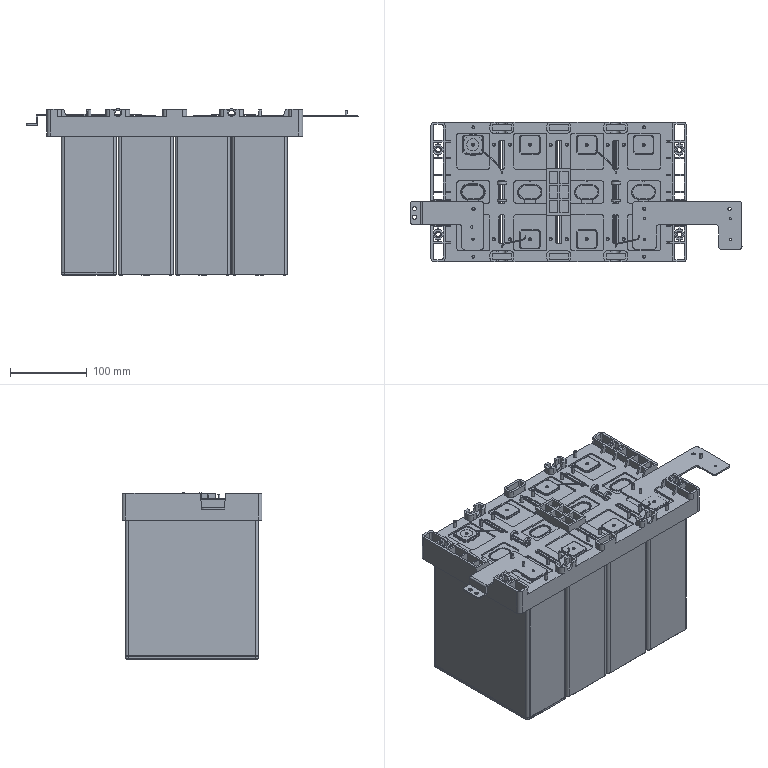Part | NX | features BREP 21 | 21 solids | 2701 faces | box 431.925 x 182 x 216.365 mm | volume 10566909 mm3 | plane 1541 | cylinder 930 | cone 112 | torus 74 | spline 40 | sphere 4 | commonest cylinder face diameters 6 x182 4 x136 3 x84 2 x60 8 x54 10 x52